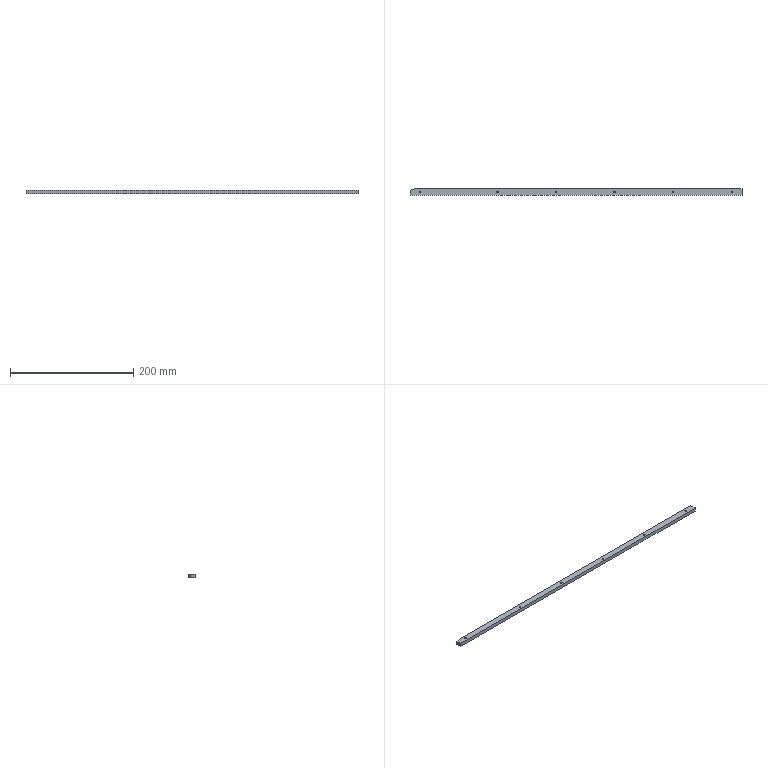Part | SolidWorks | features BaseBody 1 | 1 solid | 19 faces | box 538 x 10 x 6 mm | volume 32064 mm3 | cylinder 12 | plane 7 | commonest cylinder face diameters 2.459 x12
STEP:
#1=CARTESIAN_POINT('',(-175.111,91.468,0.));
#2=VERTEX_POINT('',#1);
#3=CARTESIAN_POINT('',(-172.652,91.468,0.));
#4=VERTEX_POINT('',#3);
#5=CARTESIAN_POINT('',(-173.881,91.468,0.));
#6=DIRECTION('',(0.,0.,1.));
#7=DIRECTION('',(1.,0.,0.));
#8=AXIS2_PLACEMENT_3D('',#5,#6,#7);
#9=CIRCLE('',#8,1.229);
#10=EDGE_CURVE('',#2,#4,#9,.T.);
#11=ORIENTED_EDGE('',*,*,#10,.F.);
#12=CARTESIAN_POINT('',(-175.111,91.468,6.));
#13=VERTEX_POINT('',#12);
#14=CARTESIAN_POINT('',(-175.111,91.468,-532.126));
#15=DIRECTION('',(0.,0.,1.));
#16=VECTOR('',#15,1000.);
#17=LINE('',#14,#16);
#18=EDGE_CURVE('',#2,#13,#17,.T.);
#19=ORIENTED_EDGE('',*,*,#18,.T.);
#20=CARTESIAN_POINT('',(-172.652,91.468,6.));
#21=VERTEX_POINT('',#20);
#22=CARTESIAN_POINT('',(-173.881,91.468,6.));
#23=DIRECTION('',(0.,0.,-1.));
#24=DIRECTION('',(1.,0.,0.));
#25=AXIS2_PLACEMENT_3D('',#22,#23,#24);
#26=CIRCLE('',#25,1.229);
#27=EDGE_CURVE('',#21,#13,#26,.T.);
#28=ORIENTED_EDGE('',*,*,#27,.F.);
#29=CARTESIAN_POINT('',(-172.652,91.468,-532.126));
#30=DIRECTION('',(0.,0.,1.));
#31=VECTOR('',#30,1000.);
#32=LINE('',#29,#31);
#33=EDGE_CURVE('',#4,#21,#32,.T.);
#34=ORIENTED_EDGE('',*,*,#33,.F.);
#35=EDGE_LOOP('',(#11,#19,#28,#34));
#36=FACE_OUTER_BOUND('',#35,.T.);
#37=CARTESIAN_POINT('',(-173.881,91.468,-532.126));
#38=DIRECTION('',(0.,0.,1.));
#39=DIRECTION('',(1.,0.,0.));
#40=AXIS2_PLACEMENT_3D('',#37,#38,#39);
#41=CYLINDRICAL_SURFACE('',#40,1.229);
#42=ADVANCED_FACE('',(#36),#41,.F.);
#43=CARTESIAN_POINT('',(-50.111,91.468,0.));
#44=VERTEX_POINT('',#43);
#45=CARTESIAN_POINT('',(-47.652,91.468,0.));
#46=VERTEX_POINT('',#45);
#47=CARTESIAN_POINT('',(-48.881,91.468,0.));
#48=DIRECTION('',(0.,0.,1.));
#49=DIRECTION('',(1.,0.,0.));
#50=AXIS2_PLACEMENT_3D('',#47,#48,#49);
#51=CIRCLE('',#50,1.23);
#52=EDGE_CURVE('',#44,#46,#51,.T.);
#53=ORIENTED_EDGE('',*,*,#52,.F.);
#54=CARTESIAN_POINT('',(-50.111,91.468,6.));
#55=VERTEX_POINT('',#54);
#56=CARTESIAN_POINT('',(-50.111,91.468,-532.126));
#57=DIRECTION('',(0.,0.,1.));
#58=VECTOR('',#57,1000.);
#59=LINE('',#56,#58);
#60=EDGE_CURVE('',#44,#55,#59,.T.);
#61=ORIENTED_EDGE('',*,*,#60,.T.);
#62=CARTESIAN_POINT('',(-47.652,91.468,6.));
#63=VERTEX_POINT('',#62);
#64=CARTESIAN_POINT('',(-48.881,91.468,6.));
#65=DIRECTION('',(0.,0.,-1.));
#66=DIRECTION('',(1.,0.,0.));
#67=AXIS2_PLACEMENT_3D('',#64,#65,#66);
#68=CIRCLE('',#67,1.23);
#69=EDGE_CURVE('',#63,#55,#68,.T.);
#70=ORIENTED_EDGE('',*,*,#69,.F.);
#71=CARTESIAN_POINT('',(-47.652,91.468,-532.126));
#72=DIRECTION('',(0.,0.,1.));
#73=VECTOR('',#72,1000.);
#74=LINE('',#71,#73);
#75=EDGE_CURVE('',#46,#63,#74,.T.);
#76=ORIENTED_EDGE('',*,*,#75,.F.);
#77=EDGE_LOOP('',(#53,#61,#70,#76));
#78=FACE_OUTER_BOUND('',#77,.T.);
#79=CARTESIAN_POINT('',(-48.881,91.468,-532.126));
#80=DIRECTION('',(0.,0.,1.));
#81=DIRECTION('',(1.,0.,0.));
#82=AXIS2_PLACEMENT_3D('',#79,#80,#81);
#83=CYLINDRICAL_SURFACE('',#82,1.23);
#84=ADVANCED_FACE('',(#78),#83,.F.);
#85=CARTESIAN_POINT('',(44.889,91.468,0.));
#86=VERTEX_POINT('',#85);
#87=CARTESIAN_POINT('',(47.348,91.468,0.));
#88=VERTEX_POINT('',#87);
#89=CARTESIAN_POINT('',(46.119,91.468,0.));
#90=DIRECTION('',(0.,0.,1.));
#91=DIRECTION('',(1.,0.,0.));
#92=AXIS2_PLACEMENT_3D('',#89,#90,#91);
#93=CIRCLE('',#92,1.23);
#94=EDGE_CURVE('',#86,#88,#93,.T.);
#95=ORIENTED_EDGE('',*,*,#94,.F.);
#96=CARTESIAN_POINT('',(44.889,91.468,6.));
#97=VERTEX_POINT('',#96);
#98=CARTESIAN_POINT('',(44.889,91.468,-532.126));
#99=DIRECTION('',(0.,0.,1.));
#100=VECTOR('',#99,1000.);
#101=LINE('',#98,#100);
#102=EDGE_CURVE('',#86,#97,#101,.T.);
#103=ORIENTED_EDGE('',*,*,#102,.T.);
#104=CARTESIAN_POINT('',(47.348,91.468,6.));
#105=VERTEX_POINT('',#104);
#106=CARTESIAN_POINT('',(46.119,91.468,6.));
#107=DIRECTION('',(0.,0.,-1.));
#108=DIRECTION('',(1.,0.,0.));
#109=AXIS2_PLACEMENT_3D('',#106,#107,#108);
#110=CIRCLE('',#109,1.23);
#111=EDGE_CURVE('',#105,#97,#110,.T.);
#112=ORIENTED_EDGE('',*,*,#111,.F.);
#113=CARTESIAN_POINT('',(47.348,91.468,-532.126));
#114=DIRECTION('',(0.,0.,1.));
#115=VECTOR('',#114,1000.);
#116=LINE('',#113,#115);
#117=EDGE_CURVE('',#88,#105,#116,.T.);
#118=ORIENTED_EDGE('',*,*,#117,.F.);
#119=EDGE_LOOP('',(#95,#103,#112,#118));
#120=FACE_OUTER_BOUND('',#119,.T.);
#121=CARTESIAN_POINT('',(46.119,91.468,-532.126));
#122=DIRECTION('',(0.,0.,1.));
#123=DIRECTION('',(1.,0.,0.));
#124=AXIS2_PLACEMENT_3D('',#121,#122,#123);
#125=CYLINDRICAL_SURFACE('',#124,1.23);
#126=ADVANCED_FACE('',(#120),#125,.F.);
#127=CARTESIAN_POINT('',(139.889,91.468,0.));
#128=VERTEX_POINT('',#127);
#129=CARTESIAN_POINT('',(142.348,91.468,0.));
#130=VERTEX_POINT('',#129);
#131=CARTESIAN_POINT('',(141.119,91.468,0.));
#132=DIRECTION('',(0.,0.,1.));
#133=DIRECTION('',(1.,0.,0.));
#134=AXIS2_PLACEMENT_3D('',#131,#132,#133);
#135=CIRCLE('',#134,1.229);
#136=EDGE_CURVE('',#128,#130,#135,.T.);
#137=ORIENTED_EDGE('',*,*,#136,.F.);
#138=CARTESIAN_POINT('',(139.889,91.468,6.));
#139=VERTEX_POINT('',#138);
#140=CARTESIAN_POINT('',(139.889,91.468,-532.126));
#141=DIRECTION('',(0.,0.,1.));
#142=VECTOR('',#141,1000.);
#143=LINE('',#140,#142);
#144=EDGE_CURVE('',#128,#139,#143,.T.);
#145=ORIENTED_EDGE('',*,*,#144,.T.);
#146=CARTESIAN_POINT('',(142.348,91.468,6.));
#147=VERTEX_POINT('',#146);
#148=CARTESIAN_POINT('',(141.119,91.468,6.));
#149=DIRECTION('',(0.,0.,-1.));
#150=DIRECTION('',(1.,0.,0.));
#151=AXIS2_PLACEMENT_3D('',#148,#149,#150);
#152=CIRCLE('',#151,1.229);
#153=EDGE_CURVE('',#147,#139,#152,.T.);
#154=ORIENTED_EDGE('',*,*,#153,.F.);
#155=CARTESIAN_POINT('',(142.348,91.468,-532.126));
#156=DIRECTION('',(0.,0.,1.));
#157=VECTOR('',#156,1000.);
#158=LINE('',#155,#157);
#159=EDGE_CURVE('',#130,#147,#158,.T.);
#160=ORIENTED_EDGE('',*,*,#159,.F.);
#161=EDGE_LOOP('',(#137,#145,#154,#160));
#162=FACE_OUTER_BOUND('',#161,.T.);
#163=CARTESIAN_POINT('',(141.119,91.468,-532.126));
#164=DIRECTION('',(0.,0.,1.));
#165=DIRECTION('',(1.,0.,0.));
#166=AXIS2_PLACEMENT_3D('',#163,#164,#165);
#167=CYLINDRICAL_SURFACE('',#166,1.229);
#168=ADVANCED_FACE('',(#162),#167,.F.);
#169=CARTESIAN_POINT('',(234.889,91.468,0.));
#170=VERTEX_POINT('',#169);
#171=CARTESIAN_POINT('',(237.348,91.468,0.));
#172=VERTEX_POINT('',#171);
#173=CARTESIAN_POINT('',(236.119,91.468,0.));
#174=DIRECTION('',(0.,0.,1.));
#175=DIRECTION('',(1.,0.,0.));
#176=AXIS2_PLACEMENT_3D('',#173,#174,#175);
#177=CIRCLE('',#176,1.229);
#178=EDGE_CURVE('',#170,#172,#177,.T.);
#179=ORIENTED_EDGE('',*,*,#178,.F.);
#180=CARTESIAN_POINT('',(234.889,91.468,6.));
#181=VERTEX_POINT('',#180);
#182=CARTESIAN_POINT('',(234.889,91.468,-532.126));
#183=DIRECTION('',(0.,0.,1.));
#184=VECTOR('',#183,1000.);
#185=LINE('',#182,#184);
#186=EDGE_CURVE('',#170,#181,#185,.T.);
#187=ORIENTED_EDGE('',*,*,#186,.T.);
#188=CARTESIAN_POINT('',(237.348,91.468,6.));
#189=VERTEX_POINT('',#188);
#190=CARTESIAN_POINT('',(236.119,91.468,6.));
#191=DIRECTION('',(0.,0.,-1.));
#192=DIRECTION('',(1.,0.,0.));
#193=AXIS2_PLACEMENT_3D('',#190,#191,#192);
#194=CIRCLE('',#193,1.229);
#195=EDGE_CURVE('',#189,#181,#194,.T.);
#196=ORIENTED_EDGE('',*,*,#195,.F.);
#197=CARTESIAN_POINT('',(237.348,91.468,-532.126));
#198=DIRECTION('',(0.,0.,1.));
#199=VECTOR('',#198,1000.);
#200=LINE('',#197,#199);
#201=EDGE_CURVE('',#172,#189,#200,.T.);
#202=ORIENTED_EDGE('',*,*,#201,.F.);
#203=EDGE_LOOP('',(#179,#187,#196,#202));
#204=FACE_OUTER_BOUND('',#203,.T.);
#205=CARTESIAN_POINT('',(236.119,91.468,-532.126));
#206=DIRECTION('',(0.,0.,1.));
#207=DIRECTION('',(1.,0.,0.));
#208=AXIS2_PLACEMENT_3D('',#205,#206,#207);
#209=CYLINDRICAL_SURFACE('',#208,1.229);
#210=ADVANCED_FACE('',(#204),#209,.F.);
#211=CARTESIAN_POINT('',(329.889,91.468,0.));
#212=VERTEX_POINT('',#211);
#213=CARTESIAN_POINT('',(332.348,91.468,0.));
#214=VERTEX_POINT('',#213);
#215=CARTESIAN_POINT('',(331.119,91.468,0.));
#216=DIRECTION('',(0.,0.,1.));
#217=DIRECTION('',(1.,0.,0.));
#218=AXIS2_PLACEMENT_3D('',#215,#216,#217);
#219=CIRCLE('',#218,1.229);
#220=EDGE_CURVE('',#212,#214,#219,.T.);
#221=ORIENTED_EDGE('',*,*,#220,.F.);
#222=CARTESIAN_POINT('',(329.889,91.468,6.));
#223=VERTEX_POINT('',#222);
#224=CARTESIAN_POINT('',(329.889,91.468,-532.126));
#225=DIRECTION('',(0.,0.,1.));
#226=VECTOR('',#225,1000.);
#227=LINE('',#224,#226);
#228=EDGE_CURVE('',#212,#223,#227,.T.);
#229=ORIENTED_EDGE('',*,*,#228,.T.);
#230=CARTESIAN_POINT('',(332.348,91.468,6.));
#231=VERTEX_POINT('',#230);
#232=CARTESIAN_POINT('',(331.119,91.468,6.));
#233=DIRECTION('',(0.,0.,-1.));
#234=DIRECTION('',(1.,0.,0.));
#235=AXIS2_PLACEMENT_3D('',#232,#233,#234);
#236=CIRCLE('',#235,1.229);
#237=EDGE_CURVE('',#231,#223,#236,.T.);
#238=ORIENTED_EDGE('',*,*,#237,.F.);
#239=CARTESIAN_POINT('',(332.348,91.468,-532.126));
#240=DIRECTION('',(0.,0.,1.));
#241=VECTOR('',#240,1000.);
#242=LINE('',#239,#241);
#243=EDGE_CURVE('',#214,#231,#242,.T.);
#244=ORIENTED_EDGE('',*,*,#243,.F.);
#245=EDGE_LOOP('',(#221,#229,#238,#244));
#246=FACE_OUTER_BOUND('',#245,.T.);
#247=CARTESIAN_POINT('',(331.119,91.468,-532.126));
#248=DIRECTION('',(0.,0.,1.));
#249=DIRECTION('',(1.,0.,0.));
#250=AXIS2_PLACEMENT_3D('',#247,#248,#249);
#251=CYLINDRICAL_SURFACE('',#250,1.229);
#252=ADVANCED_FACE('',(#246),#251,.F.);
#253=ORIENTED_EDGE('',*,*,#27,.T.);
#254=CARTESIAN_POINT('',(-173.881,91.468,6.));
#255=DIRECTION('',(0.,0.,-1.));
#256=DIRECTION('',(1.,0.,0.));
#257=AXIS2_PLACEMENT_3D('',#254,#255,#256);
#258=CIRCLE('',#257,1.229);
#259=EDGE_CURVE('',#13,#21,#258,.T.);
#260=ORIENTED_EDGE('',*,*,#259,.T.);
#261=EDGE_LOOP('',(#253,#260));
#262=FACE_BOUND('',#261,.T.);
#263=ORIENTED_EDGE('',*,*,#69,.T.);
#264=CARTESIAN_POINT('',(-48.881,91.468,6.));
#265=DIRECTION('',(0.,0.,-1.));
#266=DIRECTION('',(1.,0.,0.));
#267=AXIS2_PLACEMENT_3D('',#264,#265,#266);
#268=CIRCLE('',#267,1.23);
#269=EDGE_CURVE('',#55,#63,#268,.T.);
#270=ORIENTED_EDGE('',*,*,#269,.T.);
#271=EDGE_LOOP('',(#263,#270));
#272=FACE_BOUND('',#271,.T.);
#273=ORIENTED_EDGE('',*,*,#111,.T.);
#274=CARTESIAN_POINT('',(46.119,91.468,6.));
#275=DIRECTION('',(0.,0.,-1.));
#276=DIRECTION('',(1.,0.,0.));
#277=AXIS2_PLACEMENT_3D('',#274,#275,#276);
#278=CIRCLE('',#277,1.23);
#279=EDGE_CURVE('',#97,#105,#278,.T.);
#280=ORIENTED_EDGE('',*,*,#279,.T.);
#281=EDGE_LOOP('',(#273,#280));
#282=FACE_BOUND('',#281,.T.);
#283=ORIENTED_EDGE('',*,*,#153,.T.);
#284=CARTESIAN_POINT('',(141.119,91.468,6.));
#285=DIRECTION('',(0.,0.,-1.));
#286=DIRECTION('',(1.,0.,0.));
#287=AXIS2_PLACEMENT_3D('',#284,#285,#286);
#288=CIRCLE('',#287,1.229);
#289=EDGE_CURVE('',#139,#147,#288,.T.);
#290=ORIENTED_EDGE('',*,*,#289,.T.);
#291=EDGE_LOOP('',(#283,#290));
#292=FACE_BOUND('',#291,.T.);
#293=ORIENTED_EDGE('',*,*,#195,.T.);
#294=CARTESIAN_POINT('',(236.119,91.468,6.));
#295=DIRECTION('',(0.,0.,-1.));
#296=DIRECTION('',(1.,0.,0.));
#297=AXIS2_PLACEMENT_3D('',#294,#295,#296);
#298=CIRCLE('',#297,1.229);
#299=EDGE_CURVE('',#181,#189,#298,.T.);
#300=ORIENTED_EDGE('',*,*,#299,.T.);
#301=EDGE_LOOP('',(#293,#300));
#302=FACE_BOUND('',#301,.T.);
#303=ORIENTED_EDGE('',*,*,#237,.T.);
#304=CARTESIAN_POINT('',(331.119,91.468,6.));
#305=DIRECTION('',(0.,0.,-1.));
#306=DIRECTION('',(1.,0.,0.));
#307=AXIS2_PLACEMENT_3D('',#304,#305,#306);
#308=CIRCLE('',#307,1.229);
#309=EDGE_CURVE('',#223,#231,#308,.T.);
#310=ORIENTED_EDGE('',*,*,#309,.T.);
#311=EDGE_LOOP('',(#303,#310));
#312=FACE_BOUND('',#311,.T.);
#313=CARTESIAN_POINT('',(347.619,86.468,6.));
#314=VERTEX_POINT('',#313);
#315=CARTESIAN_POINT('',(347.619,96.468,6.));
#316=VERTEX_POINT('',#315);
#317=CARTESIAN_POINT('',(347.619,91.468,6.));
#318=DIRECTION('',(0.,1.,0.));
#319=VECTOR('',#318,1000.);
#320=LINE('',#317,#319);
#321=EDGE_CURVE('',#314,#316,#320,.T.);
#322=ORIENTED_EDGE('',*,*,#321,.T.);
#323=CARTESIAN_POINT('',(-182.881,96.468,6.));
#324=VERTEX_POINT('',#323);
#325=CARTESIAN_POINT('',(78.619,96.468,6.));
#326=DIRECTION('',(-1.,0.,0.));
#327=VECTOR('',#326,1000.);
#328=LINE('',#325,#327);
#329=EDGE_CURVE('',#316,#324,#328,.T.);
#330=ORIENTED_EDGE('',*,*,#329,.T.);
#331=CARTESIAN_POINT('',(-190.381,94.468,6.));
#332=VERTEX_POINT('',#331);
#333=CARTESIAN_POINT('',(-182.881,96.468,6.));
#334=DIRECTION('',(-0.9662,-0.2577,0.));
#335=VECTOR('',#334,1000.);
#336=LINE('',#333,#335);
#337=EDGE_CURVE('',#324,#332,#336,.T.);
#338=ORIENTED_EDGE('',*,*,#337,.T.);
#339=CARTESIAN_POINT('',(-190.381,86.468,6.));
#340=VERTEX_POINT('',#339);
#341=CARTESIAN_POINT('',(-190.381,91.468,6.));
#342=DIRECTION('',(0.,-1.,0.));
#343=VECTOR('',#342,1000.);
#344=LINE('',#341,#343);
#345=EDGE_CURVE('',#332,#340,#344,.T.);
#346=ORIENTED_EDGE('',*,*,#345,.T.);
#347=CARTESIAN_POINT('',(78.619,86.468,6.));
#348=DIRECTION('',(1.,0.,0.));
#349=VECTOR('',#348,1000.);
#350=LINE('',#347,#349);
#351=EDGE_CURVE('',#340,#314,#350,.T.);
#352=ORIENTED_EDGE('',*,*,#351,.T.);
#353=EDGE_LOOP('',(#322,#330,#338,#346,#352));
#354=FACE_OUTER_BOUND('',#353,.T.);
#355=CARTESIAN_POINT('',(78.619,91.468,6.));
#356=DIRECTION('',(0.,0.,1.));
#357=DIRECTION('',(1.,0.,0.));
#358=AXIS2_PLACEMENT_3D('',#355,#356,#357);
#359=PLANE('',#358);
#360=ADVANCED_FACE('',(#262,#272,#282,#292,#302,#312,#354),#359,.T.);
#361=ORIENTED_EDGE('',*,*,#18,.F.);
#362=CARTESIAN_POINT('',(-173.881,91.468,0.));
#363=DIRECTION('',(0.,0.,1.));
#364=DIRECTION('',(1.,0.,0.));
#365=AXIS2_PLACEMENT_3D('',#362,#363,#364);
#366=CIRCLE('',#365,1.229);
#367=EDGE_CURVE('',#4,#2,#366,.T.);
#368=ORIENTED_EDGE('',*,*,#367,.F.);
#369=ORIENTED_EDGE('',*,*,#33,.T.);
#370=ORIENTED_EDGE('',*,*,#259,.F.);
#371=EDGE_LOOP('',(#361,#368,#369,#370));
#372=FACE_OUTER_BOUND('',#371,.T.);
#373=CARTESIAN_POINT('',(-173.881,91.468,-532.126));
#374=DIRECTION('',(0.,0.,1.));
#375=DIRECTION('',(1.,0.,0.));
#376=AXIS2_PLACEMENT_3D('',#373,#374,#375);
#377=CYLINDRICAL_SURFACE('',#376,1.229);
#378=ADVANCED_FACE('',(#372),#377,.F.);
#379=ORIENTED_EDGE('',*,*,#60,.F.);
#380=CARTESIAN_POINT('',(-48.881,91.468,0.));
#381=DIRECTION('',(0.,0.,1.));
#382=DIRECTION('',(1.,0.,0.));
#383=AXIS2_PLACEMENT_3D('',#380,#381,#382);
#384=CIRCLE('',#383,1.23);
#385=EDGE_CURVE('',#46,#44,#384,.T.);
#386=ORIENTED_EDGE('',*,*,#385,.F.);
#387=ORIENTED_EDGE('',*,*,#75,.T.);
#388=ORIENTED_EDGE('',*,*,#269,.F.);
#389=EDGE_LOOP('',(#379,#386,#387,#388));
#390=FACE_OUTER_BOUND('',#389,.T.);
#391=CARTESIAN_POINT('',(-48.881,91.468,-532.126));
#392=DIRECTION('',(0.,0.,1.));
#393=DIRECTION('',(1.,0.,0.));
#394=AXIS2_PLACEMENT_3D('',#391,#392,#393);
#395=CYLINDRICAL_SURFACE('',#394,1.23);
#396=ADVANCED_FACE('',(#390),#395,.F.);
#397=ORIENTED_EDGE('',*,*,#102,.F.);
#398=CARTESIAN_POINT('',(46.119,91.468,0.));
#399=DIRECTION('',(0.,0.,1.));
#400=DIRECTION('',(1.,0.,0.));
#401=AXIS2_PLACEMENT_3D('',#398,#399,#400);
#402=CIRCLE('',#401,1.23);
#403=EDGE_CURVE('',#88,#86,#402,.T.);
#404=ORIENTED_EDGE('',*,*,#403,.F.);
#405=ORIENTED_EDGE('',*,*,#117,.T.);
#406=ORIENTED_EDGE('',*,*,#279,.F.);
#407=EDGE_LOOP('',(#397,#404,#405,#406));
#408=FACE_OUTER_BOUND('',#407,.T.);
#409=CARTESIAN_POINT('',(46.119,91.468,-532.126));
#410=DIRECTION('',(0.,0.,1.));
#411=DIRECTION('',(1.,0.,0.));
#412=AXIS2_PLACEMENT_3D('',#409,#410,#411);
#413=CYLINDRICAL_SURFACE('',#412,1.23);
#414=ADVANCED_FACE('',(#408),#413,.F.);
#415=ORIENTED_EDGE('',*,*,#144,.F.);
#416=CARTESIAN_POINT('',(141.119,91.468,0.));
#417=DIRECTION('',(0.,0.,1.));
#418=DIRECTION('',(1.,0.,0.));
#419=AXIS2_PLACEMENT_3D('',#416,#417,#418);
#420=CIRCLE('',#419,1.229);
#421=EDGE_CURVE('',#130,#128,#420,.T.);
#422=ORIENTED_EDGE('',*,*,#421,.F.);
#423=ORIENTED_EDGE('',*,*,#159,.T.);
#424=ORIENTED_EDGE('',*,*,#289,.F.);
#425=EDGE_LOOP('',(#415,#422,#423,#424));
#426=FACE_OUTER_BOUND('',#425,.T.);
#427=CARTESIAN_POINT('',(141.119,91.468,-532.126));
#428=DIRECTION('',(0.,0.,1.));
#429=DIRECTION('',(1.,0.,0.));
#430=AXIS2_PLACEMENT_3D('',#427,#428,#429);
#431=CYLINDRICAL_SURFACE('',#430,1.229);
#432=ADVANCED_FACE('',(#426),#431,.F.);
#433=ORIENTED_EDGE('',*,*,#186,.F.);
#434=CARTESIAN_POINT('',(236.119,91.468,0.));
#435=DIRECTION('',(0.,0.,1.));
#436=DIRECTION('',(1.,0.,0.));
#437=AXIS2_PLACEMENT_3D('',#434,#435,#436);
#438=CIRCLE('',#437,1.229);
#439=EDGE_CURVE('',#172,#170,#438,.T.);
#440=ORIENTED_EDGE('',*,*,#439,.F.);
#441=ORIENTED_EDGE('',*,*,#201,.T.);
#442=ORIENTED_EDGE('',*,*,#299,.F.);
#443=EDGE_LOOP('',(#433,#440,#441,#442));
#444=FACE_OUTER_BOUND('',#443,.T.);
#445=CARTESIAN_POINT('',(236.119,91.468,-532.126));
#446=DIRECTION('',(0.,0.,1.));
#447=DIRECTION('',(1.,0.,0.));
#448=AXIS2_PLACEMENT_3D('',#445,#446,#447);
#449=CYLINDRICAL_SURFACE('',#448,1.229);
#450=ADVANCED_FACE('',(#444),#449,.F.);
#451=ORIENTED_EDGE('',*,*,#228,.F.);
#452=CARTESIAN_POINT('',(331.119,91.468,0.));
#453=DIRECTION('',(0.,0.,1.));
#454=DIRECTION('',(1.,0.,0.));
#455=AXIS2_PLACEMENT_3D('',#452,#453,#454);
#456=CIRCLE('',#455,1.229);
#457=EDGE_CURVE('',#214,#212,#456,.T.);
#458=ORIENTED_EDGE('',*,*,#457,.F.);
#459=ORIENTED_EDGE('',*,*,#243,.T.);
#460=ORIENTED_EDGE('',*,*,#309,.F.);
#461=EDGE_LOOP('',(#451,#458,#459,#460));
#462=FACE_OUTER_BOUND('',#461,.T.);
#463=CARTESIAN_POINT('',(331.119,91.468,-532.126));
#464=DIRECTION('',(0.,0.,1.));
#465=DIRECTION('',(1.,0.,0.));
#466=AXIS2_PLACEMENT_3D('',#463,#464,#465);
#467=CYLINDRICAL_SURFACE('',#466,1.229);
#468=ADVANCED_FACE('',(#462),#467,.F.);
#469=CARTESIAN_POINT('',(347.619,96.468,0.));
#470=VERTEX_POINT('',#469);
#471=CARTESIAN_POINT('',(347.619,96.468,0.));
#472=DIRECTION('',(0.,0.,-1.));
#473=VECTOR('',#472,1000.);
#474=LINE('',#471,#473);
#475=EDGE_CURVE('',#316,#470,#474,.T.);
#476=ORIENTED_EDGE('',*,*,#475,.T.);
#477=CARTESIAN_POINT('',(-182.881,96.468,0.));
#478=VERTEX_POINT('',#477);
#479=CARTESIAN_POINT('',(-190.381,96.468,0.));
#480=DIRECTION('',(-1.,0.,0.));
#481=VECTOR('',#480,1000.);
#482=LINE('',#479,#481);
#483=EDGE_CURVE('',#470,#478,#482,.T.);
#484=ORIENTED_EDGE('',*,*,#483,.T.);
#485=CARTESIAN_POINT('',(-182.881,96.468,0.));
#486=DIRECTION('',(0.,0.,1.));
#487=VECTOR('',#486,1000.);
#488=LINE('',#485,#487);
#489=EDGE_CURVE('',#478,#324,#488,.T.);
#490=ORIENTED_EDGE('',*,*,#489,.T.);
#491=ORIENTED_EDGE('',*,*,#329,.F.);
#492=EDGE_LOOP('',(#476,#484,#490,#491));
#493=FACE_OUTER_BOUND('',#492,.T.);
#494=CARTESIAN_POINT('',(-190.381,96.468,0.));
#495=DIRECTION('',(0.,1.,0.));
#496=DIRECTION('',(0.,0.,1.));
#497=AXIS2_PLACEMENT_3D('',#494,#495,#496);
#498=PLANE('',#497);
#499=ADVANCED_FACE('',(#493),#498,.T.);
#500=CARTESIAN_POINT('',(347.619,86.468,0.));
#501=VERTEX_POINT('',#500);
#502=CARTESIAN_POINT('',(347.619,96.468,0.));
#503=DIRECTION('',(0.,1.,0.));
#504=VECTOR('',#503,1000.);
#505=LINE('',#502,#504);
#506=EDGE_CURVE('',#501,#470,#505,.T.);
#507=ORIENTED_EDGE('',*,*,#506,.T.);
#508=ORIENTED_EDGE('',*,*,#475,.F.);
#509=ORIENTED_EDGE('',*,*,#321,.F.);
#510=CARTESIAN_POINT('',(347.619,86.468,0.));
#511=DIRECTION('',(0.,0.,-1.));
#512=VECTOR('',#511,1000.);
#513=LINE('',#510,#512);
#514=EDGE_CURVE('',#314,#501,#513,.T.);
#515=ORIENTED_EDGE('',*,*,#514,.T.);
#516=EDGE_LOOP('',(#507,#508,#509,#515));
#517=FACE_OUTER_BOUND('',#516,.T.);
#518=CARTESIAN_POINT('',(347.619,96.468,0.));
#519=DIRECTION('',(1.,0.,0.));
#520=DIRECTION('',(0.,0.,-1.));
#521=AXIS2_PLACEMENT_3D('',#518,#519,#520);
#522=PLANE('',#521);
#523=ADVANCED_FACE('',(#517),#522,.T.);
#524=CARTESIAN_POINT('',(-190.381,86.468,0.));
#525=VERTEX_POINT('',#524);
#526=CARTESIAN_POINT('',(347.619,86.468,0.));
#527=DIRECTION('',(1.,0.,0.));
#528=VECTOR('',#527,1000.);
#529=LINE('',#526,#528);
#530=EDGE_CURVE('',#525,#501,#529,.T.);
#531=ORIENTED_EDGE('',*,*,#530,.T.);
#532=ORIENTED_EDGE('',*,*,#514,.F.);
#533=ORIENTED_EDGE('',*,*,#351,.F.);
#534=CARTESIAN_POINT('',(-190.381,86.468,0.));
#535=DIRECTION('',(0.,0.,-1.));
#536=VECTOR('',#535,1000.);
#537=LINE('',#534,#536);
#538=EDGE_CURVE('',#340,#525,#537,.T.);
#539=ORIENTED_EDGE('',*,*,#538,.T.);
#540=EDGE_LOOP('',(#531,#532,#533,#539));
#541=FACE_OUTER_BOUND('',#540,.T.);
#542=CARTESIAN_POINT('',(347.619,86.468,0.));
#543=DIRECTION('',(0.,-1.,0.));
#544=DIRECTION('',(0.,0.,-1.));
#545=AXIS2_PLACEMENT_3D('',#542,#543,#544);
#546=PLANE('',#545);
#547=ADVANCED_FACE('',(#541),#546,.T.);
#548=ORIENTED_EDGE('',*,*,#538,.F.);
#549=ORIENTED_EDGE('',*,*,#345,.F.);
#550=CARTESIAN_POINT('',(-190.381,94.468,0.));
#551=VERTEX_POINT('',#550);
#552=CARTESIAN_POINT('',(-190.381,94.468,0.));
#553=DIRECTION('',(0.,0.,-1.));
#554=VECTOR('',#553,1000.);
#555=LINE('',#552,#554);
#556=EDGE_CURVE('',#332,#551,#555,.T.);
#557=ORIENTED_EDGE('',*,*,#556,.T.);
#558=CARTESIAN_POINT('',(-190.381,86.468,0.));
#559=DIRECTION('',(0.,-1.,0.));
#560=VECTOR('',#559,1000.);
#561=LINE('',#558,#560);
#562=EDGE_CURVE('',#551,#525,#561,.T.);
#563=ORIENTED_EDGE('',*,*,#562,.T.);
#564=EDGE_LOOP('',(#548,#549,#557,#563));
#565=FACE_OUTER_BOUND('',#564,.T.);
#566=CARTESIAN_POINT('',(-190.381,86.468,0.));
#567=DIRECTION('',(-1.,0.,0.));
#568=DIRECTION('',(0.,0.,1.));
#569=AXIS2_PLACEMENT_3D('',#566,#567,#568);
#570=PLANE('',#569);
#571=ADVANCED_FACE('',(#565),#570,.T.);
#572=CARTESIAN_POINT('',(-186.631,95.468,0.));
#573=DIRECTION('',(-0.9662,-0.2577,0.));
#574=VECTOR('',#573,1000.);
#575=LINE('',#572,#574);
#576=EDGE_CURVE('',#478,#551,#575,.T.);
#577=ORIENTED_EDGE('',*,*,#576,.T.);
#578=ORIENTED_EDGE('',*,*,#556,.F.);
#579=ORIENTED_EDGE('',*,*,#337,.F.);
#580=ORIENTED_EDGE('',*,*,#489,.F.);
#581=EDGE_LOOP('',(#577,#578,#579,#580));
#582=FACE_OUTER_BOUND('',#581,.T.);
#583=CARTESIAN_POINT('',(-186.631,95.468,0.));
#584=DIRECTION('',(-0.2577,0.9662,0.));
#585=DIRECTION('',(-0.9662,-0.2577,0.));
#586=AXIS2_PLACEMENT_3D('',#583,#584,#585);
#587=PLANE('',#586);
#588=ADVANCED_FACE('',(#582),#587,.T.);
#589=ORIENTED_EDGE('',*,*,#457,.T.);
#590=ORIENTED_EDGE('',*,*,#220,.T.);
#591=EDGE_LOOP('',(#589,#590));
#592=FACE_BOUND('',#591,.T.);
#593=ORIENTED_EDGE('',*,*,#439,.T.);
#594=ORIENTED_EDGE('',*,*,#178,.T.);
#595=EDGE_LOOP('',(#593,#594));
#596=FACE_BOUND('',#595,.T.);
#597=ORIENTED_EDGE('',*,*,#421,.T.);
#598=ORIENTED_EDGE('',*,*,#136,.T.);
#599=EDGE_LOOP('',(#597,#598));
#600=FACE_BOUND('',#599,.T.);
#601=ORIENTED_EDGE('',*,*,#403,.T.);
#602=ORIENTED_EDGE('',*,*,#94,.T.);
#603=EDGE_LOOP('',(#601,#602));
#604=FACE_BOUND('',#603,.T.);
#605=ORIENTED_EDGE('',*,*,#385,.T.);
#606=ORIENTED_EDGE('',*,*,#52,.T.);
#607=EDGE_LOOP('',(#605,#606));
#608=FACE_BOUND('',#607,.T.);
#609=ORIENTED_EDGE('',*,*,#367,.T.);
#610=ORIENTED_EDGE('',*,*,#10,.T.);
#611=EDGE_LOOP('',(#609,#610));
#612=FACE_BOUND('',#611,.T.);
#613=ORIENTED_EDGE('',*,*,#483,.F.);
#614=ORIENTED_EDGE('',*,*,#506,.F.);
#615=ORIENTED_EDGE('',*,*,#530,.F.);
#616=ORIENTED_EDGE('',*,*,#562,.F.);
#617=ORIENTED_EDGE('',*,*,#576,.F.);
#618=EDGE_LOOP('',(#613,#614,#615,#616,#617));
#619=FACE_OUTER_BOUND('',#618,.T.);
#620=CARTESIAN_POINT('',(78.619,91.468,0.));
#621=DIRECTION('',(0.,0.,1.));
#622=DIRECTION('',(1.,0.,0.));
#623=AXIS2_PLACEMENT_3D('',#620,#621,#622);
#624=PLANE('',#623);
#625=ADVANCED_FACE('',(#592,#596,#600,#604,#608,#612,#619),#624,.F.);
#626=CLOSED_SHELL('',(#42,#84,#126,#168,#210,#252,#360,#378,#396,#414,#432,#450,#468,#499,#523,#547,#571,#588,#625));
#627=MANIFOLD_SOLID_BREP('',#626);
#628=CARTESIAN_POINT('',(0.,0.,0.));
#629=DIRECTION('',(0.,0.,1.));
#630=DIRECTION('',(1.,0.,0.));
#631=AXIS2_PLACEMENT_3D('',#628,#629,#630);
#632=(LENGTH_UNIT()NAMED_UNIT(*)SI_UNIT(.MILLI.,.METRE.));
#633=UNCERTAINTY_MEASURE_WITH_UNIT(LENGTH_MEASURE(0.00001),#632,'','');
#634=(NAMED_UNIT(*)PLANE_ANGLE_UNIT()SI_UNIT($,.RADIAN.));
#635=(NAMED_UNIT(*)SI_UNIT($,.STERADIAN.)SOLID_ANGLE_UNIT());
#636=(GEOMETRIC_REPRESENTATION_CONTEXT(3)GLOBAL_UNCERTAINTY_ASSIGNED_CONTEXT((#633))GLOBAL_UNIT_ASSIGNED_CONTEXT((#632,#634,#635))REPRESENTATION_CONTEXT('',''));
#637=ADVANCED_BREP_SHAPE_REPRESENTATION('',(#627,#631),#636);